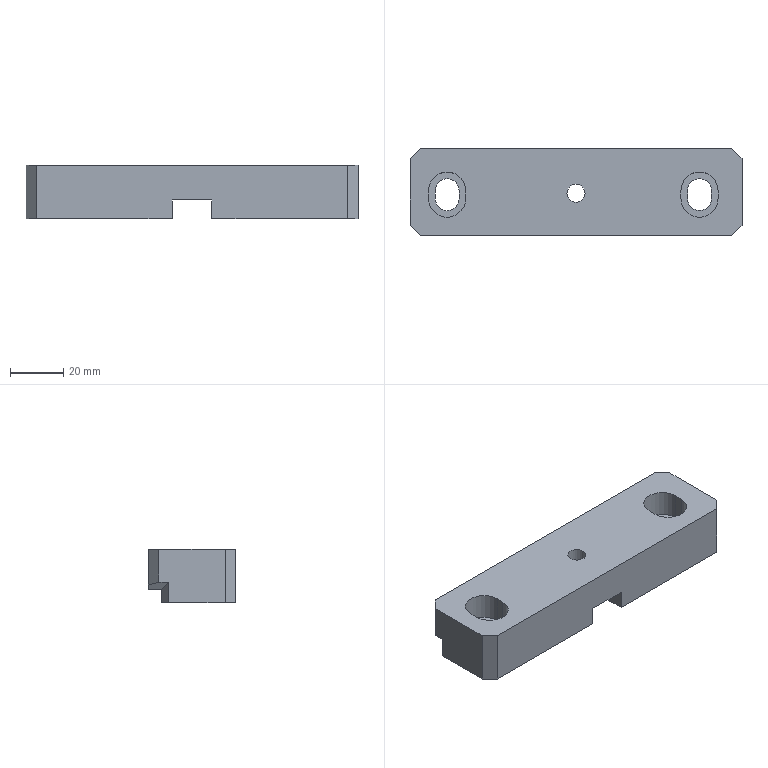Part | NX | features 20 2 | 1 solid | 46 faces | box 125 x 33 x 20 mm | volume 69012 mm3 | plane 35 | cylinder 11 | commonest cylinder face diameters 9 x4 14 x4 20 x2 6.8 x1
STEP:
#1=CARTESIAN_POINT('',(1079.502,-436.5,16.5));
#2=VERTEX_POINT('',#1);
#3=CARTESIAN_POINT('',(1079.502,-433.5,16.5));
#4=VERTEX_POINT('',#3);
#5=CARTESIAN_POINT('',(1079.502,-450.5,16.5));
#6=DIRECTION('',(0.,1.,0.));
#7=VECTOR('',#6,1000.);
#8=LINE('',#5,#7);
#9=EDGE_CURVE('',#2,#4,#8,.T.);
#10=ORIENTED_EDGE('',*,*,#9,.F.);
#11=CARTESIAN_POINT('',(1065.502,-436.5,16.5));
#12=VERTEX_POINT('',#11);
#13=CARTESIAN_POINT('',(1072.502,-436.5,16.5));
#14=DIRECTION('',(0.,0.,1.));
#15=DIRECTION('',(1.,0.,0.));
#16=AXIS2_PLACEMENT_3D('',#13,#14,#15);
#17=CIRCLE('',#16,7.);
#18=EDGE_CURVE('',#12,#2,#17,.T.);
#19=ORIENTED_EDGE('',*,*,#18,.F.);
#20=CARTESIAN_POINT('',(1065.502,-433.5,16.5));
#21=VERTEX_POINT('',#20);
#22=CARTESIAN_POINT('',(1065.502,-450.5,16.5));
#23=DIRECTION('',(0.,-1.,0.));
#24=VECTOR('',#23,1000.);
#25=LINE('',#22,#24);
#26=EDGE_CURVE('',#21,#12,#25,.T.);
#27=ORIENTED_EDGE('',*,*,#26,.F.);
#28=CARTESIAN_POINT('',(1072.502,-433.5,16.5));
#29=DIRECTION('',(0.,0.,1.));
#30=DIRECTION('',(1.,0.,0.));
#31=AXIS2_PLACEMENT_3D('',#28,#29,#30);
#32=CIRCLE('',#31,7.);
#33=EDGE_CURVE('',#4,#21,#32,.T.);
#34=ORIENTED_EDGE('',*,*,#33,.F.);
#35=EDGE_LOOP('',(#10,#19,#27,#34));
#36=FACE_BOUND('',#35,.T.);
#37=CARTESIAN_POINT('',(1183.502,-446.5,16.5));
#38=VERTEX_POINT('',#37);
#39=CARTESIAN_POINT('',(1183.502,-421.5,16.5));
#40=VERTEX_POINT('',#39);
#41=CARTESIAN_POINT('',(1183.502,-450.5,16.5));
#42=DIRECTION('',(0.,1.,0.));
#43=VECTOR('',#42,1000.);
#44=LINE('',#41,#43);
#45=EDGE_CURVE('',#38,#40,#44,.T.);
#46=ORIENTED_EDGE('',*,*,#45,.T.);
#47=CARTESIAN_POINT('',(1179.502,-417.5,16.5));
#48=VERTEX_POINT('',#47);
#49=CARTESIAN_POINT('',(1179.502,-417.5,16.5));
#50=DIRECTION('',(-0.7071,0.7071,0.));
#51=VECTOR('',#50,1000.);
#52=LINE('',#49,#51);
#53=EDGE_CURVE('',#40,#48,#52,.T.);
#54=ORIENTED_EDGE('',*,*,#53,.T.);
#55=CARTESIAN_POINT('',(1062.502,-417.5,16.5));
#56=VERTEX_POINT('',#55);
#57=CARTESIAN_POINT('',(1216.502,-417.5,16.5));
#58=DIRECTION('',(-1.,0.,0.));
#59=VECTOR('',#58,1000.);
#60=LINE('',#57,#59);
#61=EDGE_CURVE('',#48,#56,#60,.T.);
#62=ORIENTED_EDGE('',*,*,#61,.T.);
#63=CARTESIAN_POINT('',(1058.502,-421.5,16.5));
#64=VERTEX_POINT('',#63);
#65=CARTESIAN_POINT('',(1058.502,-421.5,16.5));
#66=DIRECTION('',(-0.7071,-0.7071,0.));
#67=VECTOR('',#66,1000.);
#68=LINE('',#65,#67);
#69=EDGE_CURVE('',#56,#64,#68,.T.);
#70=ORIENTED_EDGE('',*,*,#69,.T.);
#71=CARTESIAN_POINT('',(1058.502,-446.5,16.5));
#72=VERTEX_POINT('',#71);
#73=CARTESIAN_POINT('',(1058.502,-417.5,16.5));
#74=DIRECTION('',(0.,-1.,0.));
#75=VECTOR('',#74,1000.);
#76=LINE('',#73,#75);
#77=EDGE_CURVE('',#64,#72,#76,.T.);
#78=ORIENTED_EDGE('',*,*,#77,.T.);
#79=CARTESIAN_POINT('',(1062.502,-450.5,16.5));
#80=VERTEX_POINT('',#79);
#81=CARTESIAN_POINT('',(1062.502,-450.5,16.5));
#82=DIRECTION('',(0.7071,-0.7071,0.));
#83=VECTOR('',#82,1000.);
#84=LINE('',#81,#83);
#85=EDGE_CURVE('',#72,#80,#84,.T.);
#86=ORIENTED_EDGE('',*,*,#85,.T.);
#87=CARTESIAN_POINT('',(1179.502,-450.5,16.5));
#88=VERTEX_POINT('',#87);
#89=CARTESIAN_POINT('',(1136.502,-450.5,16.5));
#90=DIRECTION('',(1.,0.,0.));
#91=VECTOR('',#90,1000.);
#92=LINE('',#89,#91);
#93=EDGE_CURVE('',#80,#88,#92,.T.);
#94=ORIENTED_EDGE('',*,*,#93,.T.);
#95=CARTESIAN_POINT('',(1183.502,-446.5,16.5));
#96=DIRECTION('',(0.7071,0.7071,0.));
#97=VECTOR('',#96,1000.);
#98=LINE('',#95,#97);
#99=EDGE_CURVE('',#88,#38,#98,.T.);
#100=ORIENTED_EDGE('',*,*,#99,.T.);
#101=EDGE_LOOP('',(#46,#54,#62,#70,#78,#86,#94,#100));
#102=FACE_BOUND('',#101,.T.);
#103=CARTESIAN_POINT('',(1160.502,-433.5,16.5));
#104=VERTEX_POINT('',#103);
#105=CARTESIAN_POINT('',(1160.502,-436.5,16.5));
#106=VERTEX_POINT('',#105);
#107=CARTESIAN_POINT('',(1160.502,-450.5,16.5));
#108=DIRECTION('',(0.,-1.,0.));
#109=VECTOR('',#108,1000.);
#110=LINE('',#107,#109);
#111=EDGE_CURVE('',#104,#106,#110,.T.);
#112=ORIENTED_EDGE('',*,*,#111,.F.);
#113=CARTESIAN_POINT('',(1174.502,-433.5,16.5));
#114=VERTEX_POINT('',#113);
#115=CARTESIAN_POINT('',(1167.502,-433.5,16.5));
#116=DIRECTION('',(0.,0.,1.));
#117=DIRECTION('',(1.,0.,0.));
#118=AXIS2_PLACEMENT_3D('',#115,#116,#117);
#119=CIRCLE('',#118,7.);
#120=EDGE_CURVE('',#114,#104,#119,.T.);
#121=ORIENTED_EDGE('',*,*,#120,.F.);
#122=CARTESIAN_POINT('',(1174.502,-436.5,16.5));
#123=VERTEX_POINT('',#122);
#124=CARTESIAN_POINT('',(1174.502,-450.5,16.5));
#125=DIRECTION('',(0.,1.,0.));
#126=VECTOR('',#125,1000.);
#127=LINE('',#124,#126);
#128=EDGE_CURVE('',#123,#114,#127,.T.);
#129=ORIENTED_EDGE('',*,*,#128,.F.);
#130=CARTESIAN_POINT('',(1167.502,-436.5,16.5));
#131=DIRECTION('',(0.,0.,1.));
#132=DIRECTION('',(1.,0.,0.));
#133=AXIS2_PLACEMENT_3D('',#130,#131,#132);
#134=CIRCLE('',#133,7.);
#135=EDGE_CURVE('',#106,#123,#134,.T.);
#136=ORIENTED_EDGE('',*,*,#135,.F.);
#137=EDGE_LOOP('',(#112,#121,#129,#136));
#138=FACE_BOUND('',#137,.T.);
#139=CARTESIAN_POINT('',(1124.402,-434.5,16.5));
#140=VERTEX_POINT('',#139);
#141=CARTESIAN_POINT('',(1121.002,-434.5,16.5));
#142=DIRECTION('',(0.,0.,-1.));
#143=DIRECTION('',(1.,0.,0.));
#144=AXIS2_PLACEMENT_3D('',#141,#142,#143);
#145=CIRCLE('',#144,3.4);
#146=EDGE_CURVE('',#140,#140,#145,.T.);
#147=ORIENTED_EDGE('',*,*,#146,.T.);
#148=EDGE_LOOP('',(#147));
#149=FACE_BOUND('',#148,.T.);
#150=CARTESIAN_POINT('',(1216.502,-450.5,16.5));
#151=DIRECTION('',(0.,0.,1.));
#152=DIRECTION('',(-1.,0.,0.));
#153=AXIS2_PLACEMENT_3D('',#150,#151,#152);
#154=PLANE('',#153);
#155=ADVANCED_FACE('',(#36,#102,#138,#149),#154,.T.);
#156=CARTESIAN_POINT('',(1142.83,-427.057,-2.5));
#157=VERTEX_POINT('',#156);
#158=CARTESIAN_POINT('',(1147.07,-428.,-2.5));
#159=VERTEX_POINT('',#158);
#160=CARTESIAN_POINT('',(1147.07,-418.,-2.5));
#161=DIRECTION('',(0.,0.,1.));
#162=DIRECTION('',(1.,0.,0.));
#163=AXIS2_PLACEMENT_3D('',#160,#161,#162);
#164=CIRCLE('',#163,10.);
#165=EDGE_CURVE('',#157,#159,#164,.T.);
#166=ORIENTED_EDGE('',*,*,#165,.T.);
#167=CARTESIAN_POINT('',(1147.07,-428.,-3.5));
#168=VERTEX_POINT('',#167);
#169=CARTESIAN_POINT('',(1147.07,-428.,-43.5));
#170=DIRECTION('',(0.,0.,-1.));
#171=VECTOR('',#170,1000.);
#172=LINE('',#169,#171);
#173=EDGE_CURVE('',#159,#168,#172,.T.);
#174=ORIENTED_EDGE('',*,*,#173,.T.);
#175=CARTESIAN_POINT('',(1142.83,-427.057,-3.5));
#176=VERTEX_POINT('',#175);
#177=CARTESIAN_POINT('',(1147.07,-418.,-3.5));
#178=DIRECTION('',(0.,0.,-1.));
#179=DIRECTION('',(1.,0.,0.));
#180=AXIS2_PLACEMENT_3D('',#177,#178,#179);
#181=CIRCLE('',#180,10.);
#182=EDGE_CURVE('',#168,#176,#181,.T.);
#183=ORIENTED_EDGE('',*,*,#182,.T.);
#184=CARTESIAN_POINT('',(1142.83,-427.057,-43.5));
#185=DIRECTION('',(0.,0.,-1.));
#186=VECTOR('',#185,1000.);
#187=LINE('',#184,#186);
#188=EDGE_CURVE('',#157,#176,#187,.T.);
#189=ORIENTED_EDGE('',*,*,#188,.F.);
#190=EDGE_LOOP('',(#166,#174,#183,#189));
#191=FACE_BOUND('',#190,.T.);
#192=CARTESIAN_POINT('',(1147.07,-418.,-43.5));
#193=DIRECTION('',(0.,0.,1.));
#194=DIRECTION('',(-1.,0.,0.));
#195=AXIS2_PLACEMENT_3D('',#192,#193,#194);
#196=CYLINDRICAL_SURFACE('',#195,10.);
#197=ADVANCED_FACE('',(#191),#196,.F.);
#198=CARTESIAN_POINT('',(1133.095,-422.5,-2.5));
#199=VERTEX_POINT('',#198);
#200=CARTESIAN_POINT('',(1091.314,-402.943,-2.5));
#201=DIRECTION('',(-0.9057,0.4239,0.));
#202=VECTOR('',#201,1000.);
#203=LINE('',#200,#202);
#204=EDGE_CURVE('',#157,#199,#203,.T.);
#205=ORIENTED_EDGE('',*,*,#204,.F.);
#206=ORIENTED_EDGE('',*,*,#188,.T.);
#207=CARTESIAN_POINT('',(1133.095,-422.5,-3.5));
#208=VERTEX_POINT('',#207);
#209=CARTESIAN_POINT('',(1089.222,-401.964,-3.5));
#210=DIRECTION('',(0.9057,-0.4239,0.));
#211=VECTOR('',#210,1000.);
#212=LINE('',#209,#211);
#213=EDGE_CURVE('',#208,#176,#212,.T.);
#214=ORIENTED_EDGE('',*,*,#213,.F.);
#215=CARTESIAN_POINT('',(1133.095,-422.5,3.5));
#216=DIRECTION('',(0.,0.,-1.));
#217=VECTOR('',#216,1000.);
#218=LINE('',#215,#217);
#219=EDGE_CURVE('',#199,#208,#218,.T.);
#220=ORIENTED_EDGE('',*,*,#219,.F.);
#221=EDGE_LOOP('',(#205,#206,#214,#220));
#222=FACE_BOUND('',#221,.T.);
#223=CARTESIAN_POINT('',(1091.314,-402.943,-43.5));
#224=DIRECTION('',(-0.4239,-0.9057,0.));
#225=DIRECTION('',(-0.9057,0.4239,0.));
#226=AXIS2_PLACEMENT_3D('',#223,#224,#225);
#227=PLANE('',#226);
#228=ADVANCED_FACE('',(#222),#227,.F.);
#229=CARTESIAN_POINT('',(1183.502,-427.984,-2.5));
#230=VERTEX_POINT('',#229);
#231=CARTESIAN_POINT('',(1182.929,-428.,-2.5));
#232=VERTEX_POINT('',#231);
#233=CARTESIAN_POINT('',(1182.929,-418.,-2.5));
#234=DIRECTION('',(0.,0.,-1.));
#235=DIRECTION('',(1.,0.,0.));
#236=AXIS2_PLACEMENT_3D('',#233,#234,#235);
#237=CIRCLE('',#236,10.);
#238=EDGE_CURVE('',#230,#232,#237,.T.);
#239=ORIENTED_EDGE('',*,*,#238,.F.);
#240=CARTESIAN_POINT('',(1183.502,-427.984,-3.5));
#241=VERTEX_POINT('',#240);
#242=CARTESIAN_POINT('',(1183.502,-427.984,-43.5));
#243=DIRECTION('',(0.,0.,1.));
#244=VECTOR('',#243,1000.);
#245=LINE('',#242,#244);
#246=EDGE_CURVE('',#241,#230,#245,.T.);
#247=ORIENTED_EDGE('',*,*,#246,.F.);
#248=CARTESIAN_POINT('',(1182.929,-428.,-3.5));
#249=VERTEX_POINT('',#248);
#250=CARTESIAN_POINT('',(1182.929,-418.,-3.5));
#251=DIRECTION('',(0.,0.,1.));
#252=DIRECTION('',(1.,0.,0.));
#253=AXIS2_PLACEMENT_3D('',#250,#251,#252);
#254=CIRCLE('',#253,10.);
#255=EDGE_CURVE('',#249,#241,#254,.T.);
#256=ORIENTED_EDGE('',*,*,#255,.F.);
#257=CARTESIAN_POINT('',(1182.929,-428.,-43.5));
#258=DIRECTION('',(0.,0.,-1.));
#259=VECTOR('',#258,1000.);
#260=LINE('',#257,#259);
#261=EDGE_CURVE('',#232,#249,#260,.T.);
#262=ORIENTED_EDGE('',*,*,#261,.F.);
#263=EDGE_LOOP('',(#239,#247,#256,#262));
#264=FACE_BOUND('',#263,.T.);
#265=CARTESIAN_POINT('',(1182.929,-418.,-43.5));
#266=DIRECTION('',(0.,0.,1.));
#267=DIRECTION('',(-1.,0.,0.));
#268=AXIS2_PLACEMENT_3D('',#265,#266,#267);
#269=CYLINDRICAL_SURFACE('',#268,10.);
#270=ADVANCED_FACE('',(#264),#269,.F.);
#271=CARTESIAN_POINT('',(1163.002,-436.5,6.5));
#272=VERTEX_POINT('',#271);
#273=CARTESIAN_POINT('',(1163.002,-433.5,6.5));
#274=VERTEX_POINT('',#273);
#275=CARTESIAN_POINT('',(1163.002,-432.5,6.5));
#276=DIRECTION('',(0.,1.,0.));
#277=VECTOR('',#276,1000.);
#278=LINE('',#275,#277);
#279=EDGE_CURVE('',#272,#274,#278,.T.);
#280=ORIENTED_EDGE('',*,*,#279,.T.);
#281=CARTESIAN_POINT('',(1172.002,-433.5,6.5));
#282=VERTEX_POINT('',#281);
#283=CARTESIAN_POINT('',(1167.502,-433.5,6.5));
#284=DIRECTION('',(0.,0.,-1.));
#285=DIRECTION('',(-1.,0.,0.));
#286=AXIS2_PLACEMENT_3D('',#283,#284,#285);
#287=CIRCLE('',#286,4.5);
#288=EDGE_CURVE('',#274,#282,#287,.T.);
#289=ORIENTED_EDGE('',*,*,#288,.T.);
#290=CARTESIAN_POINT('',(1172.002,-436.5,6.5));
#291=VERTEX_POINT('',#290);
#292=CARTESIAN_POINT('',(1172.002,-439.5,6.5));
#293=DIRECTION('',(0.,-1.,0.));
#294=VECTOR('',#293,1000.);
#295=LINE('',#292,#294);
#296=EDGE_CURVE('',#282,#291,#295,.T.);
#297=ORIENTED_EDGE('',*,*,#296,.T.);
#298=CARTESIAN_POINT('',(1167.502,-436.5,6.5));
#299=DIRECTION('',(0.,0.,-1.));
#300=DIRECTION('',(-1.,0.,0.));
#301=AXIS2_PLACEMENT_3D('',#298,#299,#300);
#302=CIRCLE('',#301,4.5);
#303=EDGE_CURVE('',#291,#272,#302,.T.);
#304=ORIENTED_EDGE('',*,*,#303,.T.);
#305=EDGE_LOOP('',(#280,#289,#297,#304));
#306=FACE_BOUND('',#305,.T.);
#307=CARTESIAN_POINT('',(1174.502,-433.5,6.5));
#308=VERTEX_POINT('',#307);
#309=CARTESIAN_POINT('',(1160.502,-433.5,6.5));
#310=VERTEX_POINT('',#309);
#311=CARTESIAN_POINT('',(1167.502,-433.5,6.5));
#312=DIRECTION('',(0.,0.,1.));
#313=DIRECTION('',(-1.,0.,0.));
#314=AXIS2_PLACEMENT_3D('',#311,#312,#313);
#315=CIRCLE('',#314,7.);
#316=EDGE_CURVE('',#308,#310,#315,.T.);
#317=ORIENTED_EDGE('',*,*,#316,.T.);
#318=CARTESIAN_POINT('',(1160.502,-436.5,6.5));
#319=VERTEX_POINT('',#318);
#320=CARTESIAN_POINT('',(1160.502,-439.5,6.5));
#321=DIRECTION('',(0.,-1.,0.));
#322=VECTOR('',#321,1000.);
#323=LINE('',#320,#322);
#324=EDGE_CURVE('',#310,#319,#323,.T.);
#325=ORIENTED_EDGE('',*,*,#324,.T.);
#326=CARTESIAN_POINT('',(1174.502,-436.5,6.5));
#327=VERTEX_POINT('',#326);
#328=CARTESIAN_POINT('',(1167.502,-436.5,6.5));
#329=DIRECTION('',(0.,0.,1.));
#330=DIRECTION('',(-1.,0.,0.));
#331=AXIS2_PLACEMENT_3D('',#328,#329,#330);
#332=CIRCLE('',#331,7.);
#333=EDGE_CURVE('',#319,#327,#332,.T.);
#334=ORIENTED_EDGE('',*,*,#333,.T.);
#335=CARTESIAN_POINT('',(1174.502,-432.5,6.5));
#336=DIRECTION('',(0.,1.,0.));
#337=VECTOR('',#336,1000.);
#338=LINE('',#335,#337);
#339=EDGE_CURVE('',#327,#308,#338,.T.);
#340=ORIENTED_EDGE('',*,*,#339,.T.);
#341=EDGE_LOOP('',(#317,#325,#334,#340));
#342=FACE_BOUND('',#341,.T.);
#343=CARTESIAN_POINT('',(1167.502,-432.5,6.5));
#344=DIRECTION('',(0.,0.,-1.));
#345=DIRECTION('',(1.,0.,0.));
#346=AXIS2_PLACEMENT_3D('',#343,#344,#345);
#347=PLANE('',#346);
#348=ADVANCED_FACE('',(#306,#342),#347,.F.);
#349=CARTESIAN_POINT('',(1077.002,-433.5,6.5));
#350=VERTEX_POINT('',#349);
#351=CARTESIAN_POINT('',(1077.002,-436.5,6.5));
#352=VERTEX_POINT('',#351);
#353=CARTESIAN_POINT('',(1077.002,-432.5,6.5));
#354=DIRECTION('',(0.,-1.,0.));
#355=VECTOR('',#354,1000.);
#356=LINE('',#353,#355);
#357=EDGE_CURVE('',#350,#352,#356,.T.);
#358=ORIENTED_EDGE('',*,*,#357,.T.);
#359=CARTESIAN_POINT('',(1068.002,-436.5,6.5));
#360=VERTEX_POINT('',#359);
#361=CARTESIAN_POINT('',(1072.502,-436.5,6.5));
#362=DIRECTION('',(0.,0.,-1.));
#363=DIRECTION('',(-1.,0.,0.));
#364=AXIS2_PLACEMENT_3D('',#361,#362,#363);
#365=CIRCLE('',#364,4.5);
#366=EDGE_CURVE('',#352,#360,#365,.T.);
#367=ORIENTED_EDGE('',*,*,#366,.T.);
#368=CARTESIAN_POINT('',(1068.002,-433.5,6.5));
#369=VERTEX_POINT('',#368);
#370=CARTESIAN_POINT('',(1068.002,-439.5,6.5));
#371=DIRECTION('',(0.,1.,0.));
#372=VECTOR('',#371,1000.);
#373=LINE('',#370,#372);
#374=EDGE_CURVE('',#360,#369,#373,.T.);
#375=ORIENTED_EDGE('',*,*,#374,.T.);
#376=CARTESIAN_POINT('',(1072.502,-433.5,6.5));
#377=DIRECTION('',(0.,0.,-1.));
#378=DIRECTION('',(-1.,0.,0.));
#379=AXIS2_PLACEMENT_3D('',#376,#377,#378);
#380=CIRCLE('',#379,4.5);
#381=EDGE_CURVE('',#369,#350,#380,.T.);
#382=ORIENTED_EDGE('',*,*,#381,.T.);
#383=EDGE_LOOP('',(#358,#367,#375,#382));
#384=FACE_BOUND('',#383,.T.);
#385=CARTESIAN_POINT('',(1079.502,-433.5,6.5));
#386=VERTEX_POINT('',#385);
#387=CARTESIAN_POINT('',(1065.502,-433.5,6.5));
#388=VERTEX_POINT('',#387);
#389=CARTESIAN_POINT('',(1072.502,-433.5,6.5));
#390=DIRECTION('',(0.,0.,1.));
#391=DIRECTION('',(-1.,0.,0.));
#392=AXIS2_PLACEMENT_3D('',#389,#390,#391);
#393=CIRCLE('',#392,7.);
#394=EDGE_CURVE('',#386,#388,#393,.T.);
#395=ORIENTED_EDGE('',*,*,#394,.T.);
#396=CARTESIAN_POINT('',(1065.502,-436.5,6.5));
#397=VERTEX_POINT('',#396);
#398=CARTESIAN_POINT('',(1065.502,-432.5,6.5));
#399=DIRECTION('',(0.,-1.,0.));
#400=VECTOR('',#399,1000.);
#401=LINE('',#398,#400);
#402=EDGE_CURVE('',#388,#397,#401,.T.);
#403=ORIENTED_EDGE('',*,*,#402,.T.);
#404=CARTESIAN_POINT('',(1079.502,-436.5,6.5));
#405=VERTEX_POINT('',#404);
#406=CARTESIAN_POINT('',(1072.502,-436.5,6.5));
#407=DIRECTION('',(0.,0.,1.));
#408=DIRECTION('',(-1.,0.,0.));
#409=AXIS2_PLACEMENT_3D('',#406,#407,#408);
#410=CIRCLE('',#409,7.);
#411=EDGE_CURVE('',#397,#405,#410,.T.);
#412=ORIENTED_EDGE('',*,*,#411,.T.);
#413=CARTESIAN_POINT('',(1079.502,-439.5,6.5));
#414=DIRECTION('',(0.,1.,0.));
#415=VECTOR('',#414,1000.);
#416=LINE('',#413,#415);
#417=EDGE_CURVE('',#405,#386,#416,.T.);
#418=ORIENTED_EDGE('',*,*,#417,.T.);
#419=EDGE_LOOP('',(#395,#403,#412,#418));
#420=FACE_BOUND('',#419,.T.);
#421=CARTESIAN_POINT('',(1072.502,-432.5,6.5));
#422=DIRECTION('',(0.,0.,-1.));
#423=DIRECTION('',(-1.,0.,0.));
#424=AXIS2_PLACEMENT_3D('',#421,#422,#423);
#425=PLANE('',#424);
#426=ADVANCED_FACE('',(#384,#420),#425,.F.);
#427=ORIENTED_EDGE('',*,*,#111,.T.);
#428=CARTESIAN_POINT('',(1160.502,-436.5,42.5));
#429=DIRECTION('',(0.,0.,1.));
#430=VECTOR('',#429,1000.);
#431=LINE('',#428,#430);
#432=EDGE_CURVE('',#319,#106,#431,.T.);
#433=ORIENTED_EDGE('',*,*,#432,.F.);
#434=ORIENTED_EDGE('',*,*,#324,.F.);
#435=CARTESIAN_POINT('',(1160.502,-433.5,42.5));
#436=DIRECTION('',(0.,0.,1.));
#437=VECTOR('',#436,1000.);
#438=LINE('',#435,#437);
#439=EDGE_CURVE('',#310,#104,#438,.T.);
#440=ORIENTED_EDGE('',*,*,#439,.T.);
#441=EDGE_LOOP('',(#427,#433,#434,#440));
#442=FACE_BOUND('',#441,.T.);
#443=CARTESIAN_POINT('',(1160.502,-439.5,42.5));
#444=DIRECTION('',(-1.,0.,0.));
#445=DIRECTION('',(0.,0.,-1.));
#446=AXIS2_PLACEMENT_3D('',#443,#444,#445);
#447=PLANE('',#446);
#448=ADVANCED_FACE('',(#442),#447,.F.);
#449=ORIENTED_EDGE('',*,*,#135,.T.);
#450=CARTESIAN_POINT('',(1174.502,-436.5,42.5));
#451=DIRECTION('',(0.,0.,1.));
#452=VECTOR('',#451,1000.);
#453=LINE('',#450,#452);
#454=EDGE_CURVE('',#327,#123,#453,.T.);
#455=ORIENTED_EDGE('',*,*,#454,.F.);
#456=ORIENTED_EDGE('',*,*,#333,.F.);
#457=ORIENTED_EDGE('',*,*,#432,.T.);
#458=EDGE_LOOP('',(#449,#455,#456,#457));
#459=FACE_BOUND('',#458,.T.);
#460=CARTESIAN_POINT('',(1167.502,-436.5,42.5));
#461=DIRECTION('',(0.,0.,-1.));
#462=DIRECTION('',(1.,0.,0.));
#463=AXIS2_PLACEMENT_3D('',#460,#461,#462);
#464=CYLINDRICAL_SURFACE('',#463,7.);
#465=ADVANCED_FACE('',(#459),#464,.F.);
#466=ORIENTED_EDGE('',*,*,#128,.T.);
#467=CARTESIAN_POINT('',(1174.502,-433.5,42.5));
#468=DIRECTION('',(0.,0.,1.));
#469=VECTOR('',#468,1000.);
#470=LINE('',#467,#469);
#471=EDGE_CURVE('',#308,#114,#470,.T.);
#472=ORIENTED_EDGE('',*,*,#471,.F.);
#473=ORIENTED_EDGE('',*,*,#339,.F.);
#474=ORIENTED_EDGE('',*,*,#454,.T.);
#475=EDGE_LOOP('',(#466,#472,#473,#474));
#476=FACE_BOUND('',#475,.T.);
#477=CARTESIAN_POINT('',(1174.502,-432.5,42.5));
#478=DIRECTION('',(1.,0.,0.));
#479=DIRECTION('',(0.,0.,1.));
#480=AXIS2_PLACEMENT_3D('',#477,#478,#479);
#481=PLANE('',#480);
#482=ADVANCED_FACE('',(#476),#481,.F.);
#483=ORIENTED_EDGE('',*,*,#120,.T.);
#484=ORIENTED_EDGE('',*,*,#439,.F.);
#485=ORIENTED_EDGE('',*,*,#316,.F.);
#486=ORIENTED_EDGE('',*,*,#471,.T.);
#487=EDGE_LOOP('',(#483,#484,#485,#486));
#488=FACE_BOUND('',#487,.T.);
#489=CARTESIAN_POINT('',(1167.502,-433.5,42.5));
#490=DIRECTION('',(0.,0.,-1.));
#491=DIRECTION('',(1.,0.,0.));
#492=AXIS2_PLACEMENT_3D('',#489,#490,#491);
#493=CYLINDRICAL_SURFACE('',#492,7.);
#494=ADVANCED_FACE('',(#488),#493,.F.);
#495=ORIENTED_EDGE('',*,*,#33,.T.);
#496=CARTESIAN_POINT('',(1065.502,-433.5,42.5));
#497=DIRECTION('',(0.,0.,-1.));
#498=VECTOR('',#497,1000.);
#499=LINE('',#496,#498);
#500=EDGE_CURVE('',#21,#388,#499,.T.);
#501=ORIENTED_EDGE('',*,*,#500,.T.);
#502=ORIENTED_EDGE('',*,*,#394,.F.);
#503=CARTESIAN_POINT('',(1079.502,-433.5,42.5));
#504=DIRECTION('',(0.,0.,-1.));
#505=VECTOR('',#504,1000.);
#506=LINE('',#503,#505);
#507=EDGE_CURVE('',#4,#386,#506,.T.);
#508=ORIENTED_EDGE('',*,*,#507,.F.);
#509=EDGE_LOOP('',(#495,#501,#502,#508));
#510=FACE_BOUND('',#509,.T.);
#511=CARTESIAN_POINT('',(1072.502,-433.5,42.5));
#512=DIRECTION('',(0.,0.,-1.));
#513=DIRECTION('',(-1.,0.,0.));
#514=AXIS2_PLACEMENT_3D('',#511,#512,#513);
#515=CYLINDRICAL_SURFACE('',#514,7.);
#516=ADVANCED_FACE('',(#510),#515,.F.);
#517=ORIENTED_EDGE('',*,*,#26,.T.);
#518=CARTESIAN_POINT('',(1065.502,-436.5,42.5));
#519=DIRECTION('',(0.,0.,-1.));
#520=VECTOR('',#519,1000.);
#521=LINE('',#518,#520);
#522=EDGE_CURVE('',#12,#397,#521,.T.);
#523=ORIENTED_EDGE('',*,*,#522,.T.);
#524=ORIENTED_EDGE('',*,*,#402,.F.);
#525=ORIENTED_EDGE('',*,*,#500,.F.);
#526=EDGE_LOOP('',(#517,#523,#524,#525));
#527=FACE_BOUND('',#526,.T.);
#528=CARTESIAN_POINT('',(1065.502,-432.5,42.5));
#529=DIRECTION('',(-1.,0.,0.));
#530=DIRECTION('',(0.,0.,1.));
#531=AXIS2_PLACEMENT_3D('',#528,#529,#530);
#532=PLANE('',#531);
#533=ADVANCED_FACE('',(#527),#532,.F.);
#534=ORIENTED_EDGE('',*,*,#18,.T.);
#535=CARTESIAN_POINT('',(1079.502,-436.5,42.5));
#536=DIRECTION('',(0.,0.,-1.));
#537=VECTOR('',#536,1000.);
#538=LINE('',#535,#537);
#539=EDGE_CURVE('',#2,#405,#538,.T.);
#540=ORIENTED_EDGE('',*,*,#539,.T.);
#541=ORIENTED_EDGE('',*,*,#411,.F.);
#542=ORIENTED_EDGE('',*,*,#522,.F.);
#543=EDGE_LOOP('',(#534,#540,#541,#542));
#544=FACE_BOUND('',#543,.T.);
#545=CARTESIAN_POINT('',(1072.502,-436.5,42.5));
#546=DIRECTION('',(0.,0.,-1.));
#547=DIRECTION('',(-1.,0.,0.));
#548=AXIS2_PLACEMENT_3D('',#545,#546,#547);
#549=CYLINDRICAL_SURFACE('',#548,7.);
#550=ADVANCED_FACE('',(#544),#549,.F.);
#551=ORIENTED_EDGE('',*,*,#9,.T.);
#552=ORIENTED_EDGE('',*,*,#507,.T.);
#553=ORIENTED_EDGE('',*,*,#417,.F.);
#554=ORIENTED_EDGE('',*,*,#539,.F.);
#555=EDGE_LOOP('',(#551,#552,#553,#554));
#556=FACE_BOUND('',#555,.T.);
#557=CARTESIAN_POINT('',(1079.502,-439.5,42.5));
#558=DIRECTION('',(1.,0.,0.));
#559=DIRECTION('',(0.,0.,-1.));
#560=AXIS2_PLACEMENT_3D('',#557,#558,#559);
#561=PLANE('',#560);
#562=ADVANCED_FACE('',(#556),#561,.F.);
#563=CARTESIAN_POINT('',(1183.502,-446.5,-3.5));
#564=VERTEX_POINT('',#563);
#565=CARTESIAN_POINT('',(1183.502,-450.5,-3.5));
#566=DIRECTION('',(0.,1.,0.));
#567=VECTOR('',#566,1000.);
#568=LINE('',#565,#567);
#569=EDGE_CURVE('',#564,#241,#568,.T.);
#570=ORIENTED_EDGE('',*,*,#569,.T.);
#571=ORIENTED_EDGE('',*,*,#246,.T.);
#572=CARTESIAN_POINT('',(1183.502,-425.18,-2.5));
#573=VERTEX_POINT('',#572);
#574=CARTESIAN_POINT('',(1183.502,-450.5,-2.5));
#575=DIRECTION('',(0.,1.,0.));
#576=VECTOR('',#575,1000.);
#577=LINE('',#574,#576);
#578=EDGE_CURVE('',#230,#573,#577,.T.);
#579=ORIENTED_EDGE('',*,*,#578,.T.);
#580=CARTESIAN_POINT('',(1183.502,-425.18,4.179));
#581=VERTEX_POINT('',#580);
#582=CARTESIAN_POINT('',(1183.502,-425.18,3.5));
#583=DIRECTION('',(0.,0.,-1.));
#584=VECTOR('',#583,1000.);
#585=LINE('',#582,#584);
#586=EDGE_CURVE('',#581,#573,#585,.T.);
#587=ORIENTED_EDGE('',*,*,#586,.F.);
#588=CARTESIAN_POINT('',(1183.502,-421.5,4.179));
#589=VERTEX_POINT('',#588);
#590=CARTESIAN_POINT('',(1183.502,-417.5,4.179));
#591=DIRECTION('',(0.,1.,0.));
#592=VECTOR('',#591,1000.);
#593=LINE('',#590,#592);
#594=EDGE_CURVE('',#581,#589,#593,.T.);
#595=ORIENTED_EDGE('',*,*,#594,.T.);
#596=CARTESIAN_POINT('',(1183.502,-421.5,11.5));
#597=DIRECTION('',(0.,0.,1.));
#598=VECTOR('',#597,1000.);
#599=LINE('',#596,#598);
#600=EDGE_CURVE('',#589,#40,#599,.T.);
#601=ORIENTED_EDGE('',*,*,#600,.T.);
#602=ORIENTED_EDGE('',*,*,#45,.F.);
#603=CARTESIAN_POINT('',(1183.502,-446.5,11.5));
#604=DIRECTION('',(0.,0.,-1.));
#605=VECTOR('',#604,1000.);
#606=LINE('',#603,#605);
#607=EDGE_CURVE('',#38,#564,#606,.T.);
#608=ORIENTED_EDGE('',*,*,#607,.T.);
#609=EDGE_LOOP('',(#570,#571,#579,#587,#595,#601,#602,#608));
#610=FACE_BOUND('',#609,.T.);
#611=CARTESIAN_POINT('',(1183.502,-450.5,11.5));
#612=DIRECTION('',(-1.,0.,0.));
#613=DIRECTION('',(0.,0.,-1.));
#614=AXIS2_PLACEMENT_3D('',#611,#612,#613);
#615=PLANE('',#614);
#616=ADVANCED_FACE('',(#610),#615,.F.);
#617=ORIENTED_EDGE('',*,*,#288,.F.);
#618=CARTESIAN_POINT('',(1163.002,-433.5,-3.5));
#619=VERTEX_POINT('',#618);
#620=CARTESIAN_POINT('',(1163.002,-433.5,42.5));
#621=DIRECTION('',(0.,0.,1.));
#622=VECTOR('',#621,1000.);
#623=LINE('',#620,#622);
#624=EDGE_CURVE('',#619,#274,#623,.T.);
#625=ORIENTED_EDGE('',*,*,#624,.F.);
#626=CARTESIAN_POINT('',(1172.002,-433.5,-3.5));
#627=VERTEX_POINT('',#626);
#628=CARTESIAN_POINT('',(1167.502,-433.5,-3.5));
#629=DIRECTION('',(0.,0.,1.));
#630=DIRECTION('',(1.,0.,0.));
#631=AXIS2_PLACEMENT_3D('',#628,#629,#630);
#632=CIRCLE('',#631,4.5);
#633=EDGE_CURVE('',#627,#619,#632,.T.);
#634=ORIENTED_EDGE('',*,*,#633,.F.);
#635=CARTESIAN_POINT('',(1172.002,-433.5,42.5));
#636=DIRECTION('',(0.,0.,1.));
#637=VECTOR('',#636,1000.);
#638=LINE('',#635,#637);
#639=EDGE_CURVE('',#627,#282,#638,.T.);
#640=ORIENTED_EDGE('',*,*,#639,.T.);
#641=EDGE_LOOP('',(#617,#625,#634,#640));
#642=FACE_BOUND('',#641,.T.);
#643=CARTESIAN_POINT('',(1167.502,-433.5,42.5));
#644=DIRECTION('',(0.,0.,-1.));
#645=DIRECTION('',(1.,0.,0.));
#646=AXIS2_PLACEMENT_3D('',#643,#644,#645);
#647=CYLINDRICAL_SURFACE('',#646,4.5);
#648=ADVANCED_FACE('',(#642),#647,.F.);
#649=ORIENTED_EDGE('',*,*,#296,.F.);
#650=ORIENTED_EDGE('',*,*,#639,.F.);
#651=CARTESIAN_POINT('',(1172.002,-436.5,-3.5));
#652=VERTEX_POINT('',#651);
#653=CARTESIAN_POINT('',(1172.002,-439.5,-3.5));
#654=DIRECTION('',(0.,1.,0.));
#655=VECTOR('',#654,1000.);
#656=LINE('',#653,#655);
#657=EDGE_CURVE('',#652,#627,#656,.T.);
#658=ORIENTED_EDGE('',*,*,#657,.F.);
#659=CARTESIAN_POINT('',(1172.002,-436.5,42.5));
#660=DIRECTION('',(0.,0.,1.));
#661=VECTOR('',#660,1000.);
#662=LINE('',#659,#661);
#663=EDGE_CURVE('',#652,#291,#662,.T.);
#664=ORIENTED_EDGE('',*,*,#663,.T.);
#665=EDGE_LOOP('',(#649,#650,#658,#664));
#666=FACE_BOUND('',#665,.T.);
#667=CARTESIAN_POINT('',(1172.002,-439.5,42.5));
#668=DIRECTION('',(-1.,0.,0.));
#669=DIRECTION('',(0.,0.,-1.));
#670=AXIS2_PLACEMENT_3D('',#667,#668,#669);
#671=PLANE('',#670);
#672=ADVANCED_FACE('',(#666),#671,.T.);
#673=ORIENTED_EDGE('',*,*,#303,.F.);
#674=ORIENTED_EDGE('',*,*,#663,.F.);
#675=CARTESIAN_POINT('',(1163.002,-436.5,-3.5));
#676=VERTEX_POINT('',#675);
#677=CARTESIAN_POINT('',(1167.502,-436.5,-3.5));
#678=DIRECTION('',(0.,0.,1.));
#679=DIRECTION('',(1.,0.,0.));
#680=AXIS2_PLACEMENT_3D('',#677,#678,#679);
#681=CIRCLE('',#680,4.5);
#682=EDGE_CURVE('',#676,#652,#681,.T.);
#683=ORIENTED_EDGE('',*,*,#682,.F.);
#684=CARTESIAN_POINT('',(1163.002,-436.5,42.5));
#685=DIRECTION('',(0.,0.,1.));
#686=VECTOR('',#685,1000.);
#687=LINE('',#684,#686);
#688=EDGE_CURVE('',#676,#272,#687,.T.);
#689=ORIENTED_EDGE('',*,*,#688,.T.);
#690=EDGE_LOOP('',(#673,#674,#683,#689));
#691=FACE_BOUND('',#690,.T.);
#692=CARTESIAN_POINT('',(1167.502,-436.5,42.5));
#693=DIRECTION('',(0.,0.,-1.));
#694=DIRECTION('',(1.,0.,0.));
#695=AXIS2_PLACEMENT_3D('',#692,#693,#694);
#696=CYLINDRICAL_SURFACE('',#695,4.5);
#697=ADVANCED_FACE('',(#691),#696,.F.);
#698=ORIENTED_EDGE('',*,*,#279,.F.);
#699=ORIENTED_EDGE('',*,*,#688,.F.);
#700=CARTESIAN_POINT('',(1163.002,-432.5,-3.5));
#701=DIRECTION('',(0.,-1.,0.));
#702=VECTOR('',#701,1000.);
#703=LINE('',#700,#702);
#704=EDGE_CURVE('',#619,#676,#703,.T.);
#705=ORIENTED_EDGE('',*,*,#704,.F.);
#706=ORIENTED_EDGE('',*,*,#624,.T.);
#707=EDGE_LOOP('',(#698,#699,#705,#706));
#708=FACE_BOUND('',#707,.T.);
#709=CARTESIAN_POINT('',(1163.002,-432.5,42.5));
#710=DIRECTION('',(1.,0.,0.));
#711=DIRECTION('',(0.,0.,1.));
#712=AXIS2_PLACEMENT_3D('',#709,#710,#711);
#713=PLANE('',#712);
#714=ADVANCED_FACE('',(#708),#713,.T.);
#715=CARTESIAN_POINT('',(1128.502,-422.5,1.5));
#716=VERTEX_POINT('',#715);
#717=CARTESIAN_POINT('',(1173.501,-422.5,1.5));
#718=VERTEX_POINT('',#717);
#719=CARTESIAN_POINT('',(1098.773,-422.5,1.5));
#720=DIRECTION('',(1.,0.,0.));
#721=VECTOR('',#720,1000.);
#722=LINE('',#719,#721);
#723=EDGE_CURVE('',#716,#718,#722,.T.);
#724=ORIENTED_EDGE('',*,*,#723,.T.);
#725=CARTESIAN_POINT('',(1173.501,-422.5,-2.5));
#726=VERTEX_POINT('',#725);
#727=CARTESIAN_POINT('',(1173.501,-422.5,3.5));
#728=DIRECTION('',(0.,0.,1.));
#729=VECTOR('',#728,1000.);
#730=LINE('',#727,#729);
#731=EDGE_CURVE('',#726,#718,#730,.T.);
#732=ORIENTED_EDGE('',*,*,#731,.F.);
#733=CARTESIAN_POINT('',(1116.501,-422.5,-2.5));
#734=DIRECTION('',(-1.,0.,0.));
#735=VECTOR('',#734,1000.);
#736=LINE('',#733,#735);
#737=EDGE_CURVE('',#726,#199,#736,.T.);
#738=ORIENTED_EDGE('',*,*,#737,.T.);
#739=ORIENTED_EDGE('',*,*,#219,.T.);
#740=CARTESIAN_POINT('',(1128.502,-422.5,-3.5));
#741=VERTEX_POINT('',#740);
#742=CARTESIAN_POINT('',(1116.501,-422.5,-3.5));
#743=DIRECTION('',(-1.,0.,0.));
#744=VECTOR('',#743,1000.);
#745=LINE('',#742,#744);
#746=EDGE_CURVE('',#208,#741,#745,.T.);
#747=ORIENTED_EDGE('',*,*,#746,.T.);
#748=CARTESIAN_POINT('',(1128.502,-422.5,-9.5));
#749=DIRECTION('',(0.,0.,1.));
#750=VECTOR('',#749,1000.);
#751=LINE('',#748,#750);
#752=EDGE_CURVE('',#741,#716,#751,.T.);
#753=ORIENTED_EDGE('',*,*,#752,.T.);
#754=EDGE_LOOP('',(#724,#732,#738,#739,#747,#753));
#755=FACE_BOUND('',#754,.T.);
#756=CARTESIAN_POINT('',(1116.501,-422.5,3.5));
#757=DIRECTION('',(0.,-1.,0.));
#758=DIRECTION('',(0.,0.,1.));
#759=AXIS2_PLACEMENT_3D('',#756,#757,#758);
#760=PLANE('',#759);
#761=ADVANCED_FACE('',(#755),#760,.F.);
#762=CARTESIAN_POINT('',(1128.502,-417.5,1.5));
#763=VERTEX_POINT('',#762);
#764=CARTESIAN_POINT('',(1128.502,-436.5,1.5));
#765=DIRECTION('',(0.,1.,0.));
#766=VECTOR('',#765,1000.);
#767=LINE('',#764,#766);
#768=EDGE_CURVE('',#716,#763,#767,.T.);
#769=ORIENTED_EDGE('',*,*,#768,.T.);
#770=CARTESIAN_POINT('',(1173.502,-417.5,1.5));
#771=VERTEX_POINT('',#770);
#772=CARTESIAN_POINT('',(1076.502,-417.5,1.5));
#773=DIRECTION('',(1.,0.,0.));
#774=VECTOR('',#773,1000.);
#775=LINE('',#772,#774);
#776=EDGE_CURVE('',#763,#771,#775,.T.);
#777=ORIENTED_EDGE('',*,*,#776,.T.);
#778=CARTESIAN_POINT('',(1173.502,-422.5,1.5));
#779=VERTEX_POINT('',#778);
#780=CARTESIAN_POINT('',(1173.502,-425.18,1.5));
#781=DIRECTION('',(0.,-1.,0.));
#782=VECTOR('',#781,1000.);
#783=LINE('',#780,#782);
#784=EDGE_CURVE('',#771,#779,#783,.T.);
#785=ORIENTED_EDGE('',*,*,#784,.T.);
#786=CARTESIAN_POINT('',(1183.502,-425.18,1.5));
#787=DIRECTION('',(0.9659,-0.2588,0.));
#788=VECTOR('',#787,1000.);
#789=LINE('',#786,#788);
#790=EDGE_CURVE('',#718,#779,#789,.T.);
#791=ORIENTED_EDGE('',*,*,#790,.F.);
#792=ORIENTED_EDGE('',*,*,#723,.F.);
#793=EDGE_LOOP('',(#769,#777,#785,#791,#792));
#794=FACE_BOUND('',#793,.T.);
#795=CARTESIAN_POINT('',(1148.773,-396.891,1.5));
#796=DIRECTION('',(0.,0.,-1.));
#797=DIRECTION('',(1.,0.,0.));
#798=AXIS2_PLACEMENT_3D('',#795,#796,#797);
#799=PLANE('',#798);
#800=ADVANCED_FACE('',(#794),#799,.T.);
#801=ORIENTED_EDGE('',*,*,#61,.F.);
#802=CARTESIAN_POINT('',(1179.502,-417.5,3.108));
#803=VERTEX_POINT('',#802);
#804=CARTESIAN_POINT('',(1179.502,-417.5,11.5));
#805=DIRECTION('',(0.,0.,-1.));
#806=VECTOR('',#805,1000.);
#807=LINE('',#804,#806);
#808=EDGE_CURVE('',#48,#803,#807,.T.);
#809=ORIENTED_EDGE('',*,*,#808,.T.);
#810=CARTESIAN_POINT('',(1173.502,-417.5,1.5));
#811=DIRECTION('',(-0.9659,0.,-0.2588));
#812=VECTOR('',#811,1000.);
#813=LINE('',#810,#812);
#814=EDGE_CURVE('',#803,#771,#813,.T.);
#815=ORIENTED_EDGE('',*,*,#814,.T.);
#816=ORIENTED_EDGE('',*,*,#776,.F.);
#817=CARTESIAN_POINT('',(1128.502,-417.5,3.5));
#818=VERTEX_POINT('',#817);
#819=CARTESIAN_POINT('',(1128.502,-417.5,11.5));
#820=DIRECTION('',(0.,0.,-1.));
#821=VECTOR('',#820,1000.);
#822=LINE('',#819,#821);
#823=EDGE_CURVE('',#818,#763,#822,.T.);
#824=ORIENTED_EDGE('',*,*,#823,.F.);
#825=CARTESIAN_POINT('',(1113.502,-417.5,3.5));
#826=VERTEX_POINT('',#825);
#827=CARTESIAN_POINT('',(1104.002,-417.5,3.5));
#828=DIRECTION('',(1.,0.,0.));
#829=VECTOR('',#828,1000.);
#830=LINE('',#827,#829);
#831=EDGE_CURVE('',#826,#818,#830,.T.);
#832=ORIENTED_EDGE('',*,*,#831,.F.);
#833=CARTESIAN_POINT('',(1113.502,-417.5,1.5));
#834=VERTEX_POINT('',#833);
#835=CARTESIAN_POINT('',(1113.502,-417.5,11.5));
#836=DIRECTION('',(0.,0.,1.));
#837=VECTOR('',#836,1000.);
#838=LINE('',#835,#837);
#839=EDGE_CURVE('',#834,#826,#838,.T.);
#840=ORIENTED_EDGE('',*,*,#839,.F.);
#841=CARTESIAN_POINT('',(1068.502,-417.5,1.5));
#842=VERTEX_POINT('',#841);
#843=CARTESIAN_POINT('',(1194.502,-417.5,1.5));
#844=DIRECTION('',(1.,0.,0.));
#845=VECTOR('',#844,1000.);
#846=LINE('',#843,#845);
#847=EDGE_CURVE('',#842,#834,#846,.T.);
#848=ORIENTED_EDGE('',*,*,#847,.F.);
#849=CARTESIAN_POINT('',(1062.502,-417.5,3.108));
#850=VERTEX_POINT('',#849);
#851=CARTESIAN_POINT('',(1068.502,-417.5,1.5));
#852=DIRECTION('',(-0.9659,0.,0.2588));
#853=VECTOR('',#852,1000.);
#854=LINE('',#851,#853);
#855=EDGE_CURVE('',#842,#850,#854,.T.);
#856=ORIENTED_EDGE('',*,*,#855,.T.);
#857=CARTESIAN_POINT('',(1062.502,-417.5,11.5));
#858=DIRECTION('',(0.,0.,1.));
#859=VECTOR('',#858,1000.);
#860=LINE('',#857,#859);
#861=EDGE_CURVE('',#850,#56,#860,.T.);
#862=ORIENTED_EDGE('',*,*,#861,.T.);
#863=EDGE_LOOP('',(#801,#809,#815,#816,#824,#832,#840,#848,#856,#862));
#864=FACE_BOUND('',#863,.T.);
#865=CARTESIAN_POINT('',(1216.502,-417.5,11.5));
#866=DIRECTION('',(0.,-1.,0.));
#867=DIRECTION('',(0.,0.,1.));
#868=AXIS2_PLACEMENT_3D('',#865,#866,#867);
#869=PLANE('',#868);
#870=ADVANCED_FACE('',(#864),#869,.F.);
#871=ORIENTED_EDGE('',*,*,#69,.F.);
#872=ORIENTED_EDGE('',*,*,#861,.F.);
#873=CARTESIAN_POINT('',(1058.502,-421.5,4.179));
#874=VERTEX_POINT('',#873);
#875=CARTESIAN_POINT('',(1075.554,-404.449,-0.3894));
#876=DIRECTION('',(0.6947,0.6947,-0.1862));
#877=VECTOR('',#876,1000.);
#878=LINE('',#875,#877);
#879=EDGE_CURVE('',#874,#850,#878,.T.);
#880=ORIENTED_EDGE('',*,*,#879,.F.);
#881=CARTESIAN_POINT('',(1058.502,-421.5,11.5));
#882=DIRECTION('',(0.,0.,-1.));
#883=VECTOR('',#882,1000.);
#884=LINE('',#881,#883);
#885=EDGE_CURVE('',#64,#874,#884,.T.);
#886=ORIENTED_EDGE('',*,*,#885,.F.);
#887=EDGE_LOOP('',(#871,#872,#880,#886));
#888=FACE_BOUND('',#887,.T.);
#889=CARTESIAN_POINT('',(1058.502,-421.5,11.5));
#890=DIRECTION('',(0.7071,-0.7071,0.));
#891=DIRECTION('',(0.,0.,-1.));
#892=AXIS2_PLACEMENT_3D('',#889,#890,#891);
#893=PLANE('',#892);
#894=ADVANCED_FACE('',(#888),#893,.F.);
#895=ORIENTED_EDGE('',*,*,#366,.F.);
#896=CARTESIAN_POINT('',(1077.002,-436.5,-3.5));
#897=VERTEX_POINT('',#896);
#898=CARTESIAN_POINT('',(1077.002,-436.5,42.5));
#899=DIRECTION('',(0.,0.,-1.));
#900=VECTOR('',#899,1000.);
#901=LINE('',#898,#900);
#902=EDGE_CURVE('',#352,#897,#901,.T.);
#903=ORIENTED_EDGE('',*,*,#902,.T.);
#904=CARTESIAN_POINT('',(1068.002,-436.5,-3.5));
#905=VERTEX_POINT('',#904);
#906=CARTESIAN_POINT('',(1072.502,-436.5,-3.5));
#907=DIRECTION('',(0.,0.,-1.));
#908=DIRECTION('',(1.,0.,0.));
#909=AXIS2_PLACEMENT_3D('',#906,#907,#908);
#910=CIRCLE('',#909,4.5);
#911=EDGE_CURVE('',#897,#905,#910,.T.);
#912=ORIENTED_EDGE('',*,*,#911,.T.);
#913=CARTESIAN_POINT('',(1068.002,-436.5,42.5));
#914=DIRECTION('',(0.,0.,-1.));
#915=VECTOR('',#914,1000.);
#916=LINE('',#913,#915);
#917=EDGE_CURVE('',#360,#905,#916,.T.);
#918=ORIENTED_EDGE('',*,*,#917,.F.);
#919=EDGE_LOOP('',(#895,#903,#912,#918));
#920=FACE_BOUND('',#919,.T.);
#921=CARTESIAN_POINT('',(1072.502,-436.5,42.5));
#922=DIRECTION('',(0.,0.,-1.));
#923=DIRECTION('',(-1.,0.,0.));
#924=AXIS2_PLACEMENT_3D('',#921,#922,#923);
#925=CYLINDRICAL_SURFACE('',#924,4.5);
#926=ADVANCED_FACE('',(#920),#925,.F.);
#927=ORIENTED_EDGE('',*,*,#374,.F.);
#928=ORIENTED_EDGE('',*,*,#917,.T.);
#929=CARTESIAN_POINT('',(1068.002,-433.5,-3.5));
#930=VERTEX_POINT('',#929);
#931=CARTESIAN_POINT('',(1068.002,-450.5,-3.5));
#932=DIRECTION('',(0.,1.,0.));
#933=VECTOR('',#932,1000.);
#934=LINE('',#931,#933);
#935=EDGE_CURVE('',#905,#930,#934,.T.);
#936=ORIENTED_EDGE('',*,*,#935,.T.);
#937=CARTESIAN_POINT('',(1068.002,-433.5,42.5));
#938=DIRECTION('',(0.,0.,-1.));
#939=VECTOR('',#938,1000.);
#940=LINE('',#937,#939);
#941=EDGE_CURVE('',#369,#930,#940,.T.);
#942=ORIENTED_EDGE('',*,*,#941,.F.);
#943=EDGE_LOOP('',(#927,#928,#936,#942));
#944=FACE_BOUND('',#943,.T.);
#945=CARTESIAN_POINT('',(1068.002,-439.5,42.5));
#946=DIRECTION('',(1.,0.,0.));
#947=DIRECTION('',(0.,0.,-1.));
#948=AXIS2_PLACEMENT_3D('',#945,#946,#947);
#949=PLANE('',#948);
#950=ADVANCED_FACE('',(#944),#949,.T.);
#951=ORIENTED_EDGE('',*,*,#381,.F.);
#952=ORIENTED_EDGE('',*,*,#941,.T.);
#953=CARTESIAN_POINT('',(1077.002,-433.5,-3.5));
#954=VERTEX_POINT('',#953);
#955=CARTESIAN_POINT('',(1072.502,-433.5,-3.5));
#956=DIRECTION('',(0.,0.,-1.));
#957=DIRECTION('',(1.,0.,0.));
#958=AXIS2_PLACEMENT_3D('',#955,#956,#957);
#959=CIRCLE('',#958,4.5);
#960=EDGE_CURVE('',#930,#954,#959,.T.);
#961=ORIENTED_EDGE('',*,*,#960,.T.);
#962=CARTESIAN_POINT('',(1077.002,-433.5,42.5));
#963=DIRECTION('',(0.,0.,-1.));
#964=VECTOR('',#963,1000.);
#965=LINE('',#962,#964);
#966=EDGE_CURVE('',#350,#954,#965,.T.);
#967=ORIENTED_EDGE('',*,*,#966,.F.);
#968=EDGE_LOOP('',(#951,#952,#961,#967));
#969=FACE_BOUND('',#968,.T.);
#970=CARTESIAN_POINT('',(1072.502,-433.5,42.5));
#971=DIRECTION('',(0.,0.,-1.));
#972=DIRECTION('',(-1.,0.,0.));
#973=AXIS2_PLACEMENT_3D('',#970,#971,#972);
#974=CYLINDRICAL_SURFACE('',#973,4.5);
#975=ADVANCED_FACE('',(#969),#974,.F.);
#976=ORIENTED_EDGE('',*,*,#357,.F.);
#977=ORIENTED_EDGE('',*,*,#966,.T.);
#978=CARTESIAN_POINT('',(1077.002,-450.5,-3.5));
#979=DIRECTION('',(0.,-1.,0.));
#980=VECTOR('',#979,1000.);
#981=LINE('',#978,#980);
#982=EDGE_CURVE('',#954,#897,#981,.T.);
#983=ORIENTED_EDGE('',*,*,#982,.T.);
#984=ORIENTED_EDGE('',*,*,#902,.F.);
#985=EDGE_LOOP('',(#976,#977,#983,#984));
#986=FACE_BOUND('',#985,.T.);
#987=CARTESIAN_POINT('',(1077.002,-432.5,42.5));
#988=DIRECTION('',(-1.,0.,0.));
#989=DIRECTION('',(0.,0.,1.));
#990=AXIS2_PLACEMENT_3D('',#987,#988,#989);
#991=PLANE('',#990);
#992=ADVANCED_FACE('',(#986),#991,.T.);
#993=ORIENTED_EDGE('',*,*,#77,.F.);
#994=ORIENTED_EDGE('',*,*,#885,.T.);
#995=CARTESIAN_POINT('',(1058.502,-425.179,4.179));
#996=VERTEX_POINT('',#995);
#997=CARTESIAN_POINT('',(1058.502,-425.179,4.179));
#998=DIRECTION('',(0.,-1.,0.));
#999=VECTOR('',#998,1000.);
#1000=LINE('',#997,#999);
#1001=EDGE_CURVE('',#874,#996,#1000,.T.);
#1002=ORIENTED_EDGE('',*,*,#1001,.T.);
#1003=CARTESIAN_POINT('',(1058.502,-425.179,-3.5));
#1004=VERTEX_POINT('',#1003);
#1005=CARTESIAN_POINT('',(1058.502,-425.179,3.5));
#1006=DIRECTION('',(0.,0.,-1.));
#1007=VECTOR('',#1006,1000.);
#1008=LINE('',#1005,#1007);
#1009=EDGE_CURVE('',#996,#1004,#1008,.T.);
#1010=ORIENTED_EDGE('',*,*,#1009,.T.);
#1011=CARTESIAN_POINT('',(1058.502,-446.5,-3.5));
#1012=VERTEX_POINT('',#1011);
#1013=CARTESIAN_POINT('',(1058.502,-417.5,-3.5));
#1014=DIRECTION('',(0.,-1.,0.));
#1015=VECTOR('',#1014,1000.);
#1016=LINE('',#1013,#1015);
#1017=EDGE_CURVE('',#1004,#1012,#1016,.T.);
#1018=ORIENTED_EDGE('',*,*,#1017,.T.);
#1019=CARTESIAN_POINT('',(1058.502,-446.5,11.5));
#1020=DIRECTION('',(0.,0.,1.));
#1021=VECTOR('',#1020,1000.);
#1022=LINE('',#1019,#1021);
#1023=EDGE_CURVE('',#1012,#72,#1022,.T.);
#1024=ORIENTED_EDGE('',*,*,#1023,.T.);
#1025=EDGE_LOOP('',(#993,#994,#1002,#1010,#1018,#1024));
#1026=FACE_BOUND('',#1025,.T.);
#1027=CARTESIAN_POINT('',(1058.502,-417.5,11.5));
#1028=DIRECTION('',(1.,0.,0.));
#1029=DIRECTION('',(0.,0.,1.));
#1030=AXIS2_PLACEMENT_3D('',#1027,#1028,#1029);
#1031=PLANE('',#1030);
#1032=ADVANCED_FACE('',(#1026),#1031,.F.);
#1033=ORIENTED_EDGE('',*,*,#1001,.F.);
#1034=ORIENTED_EDGE('',*,*,#879,.T.);
#1035=ORIENTED_EDGE('',*,*,#855,.F.);
#1036=CARTESIAN_POINT('',(1068.502,-422.5,1.5));
#1037=VERTEX_POINT('',#1036);
#1038=CARTESIAN_POINT('',(1068.502,-417.5,1.5));
#1039=DIRECTION('',(0.,1.,0.));
#1040=VECTOR('',#1039,1000.);
#1041=LINE('',#1038,#1040);
#1042=EDGE_CURVE('',#1037,#842,#1041,.T.);
#1043=ORIENTED_EDGE('',*,*,#1042,.F.);
#1044=CARTESIAN_POINT('',(1068.501,-422.5,1.5));
#1045=VERTEX_POINT('',#1044);
#1046=CARTESIAN_POINT('',(1068.502,-422.5,1.5));
#1047=DIRECTION('',(0.9659,0.,-0.2588));
#1048=VECTOR('',#1047,1000.);
#1049=LINE('',#1046,#1048);
#1050=EDGE_CURVE('',#1045,#1037,#1049,.T.);
#1051=ORIENTED_EDGE('',*,*,#1050,.F.);
#1052=CARTESIAN_POINT('',(1068.501,-422.5,1.5));
#1053=DIRECTION('',(0.9351,0.2506,-0.2506));
#1054=VECTOR('',#1053,1000.);
#1055=LINE('',#1052,#1054);
#1056=EDGE_CURVE('',#996,#1045,#1055,.T.);
#1057=ORIENTED_EDGE('',*,*,#1056,.F.);
#1058=EDGE_LOOP('',(#1033,#1034,#1035,#1043,#1051,#1057));
#1059=FACE_BOUND('',#1058,.T.);
#1060=CARTESIAN_POINT('',(1068.502,-396.891,1.5));
#1061=DIRECTION('',(-0.2588,0.,-0.9659));
#1062=DIRECTION('',(0.9659,0.,-0.2588));
#1063=AXIS2_PLACEMENT_3D('',#1060,#1061,#1062);
#1064=PLANE('',#1063);
#1065=ADVANCED_FACE('',(#1059),#1064,.T.);
#1066=CARTESIAN_POINT('',(1068.501,-422.5,-3.5));
#1067=VERTEX_POINT('',#1066);
#1068=CARTESIAN_POINT('',(1068.501,-422.5,-3.5));
#1069=DIRECTION('',(-0.9659,-0.2588,0.));
#1070=VECTOR('',#1069,1000.);
#1071=LINE('',#1068,#1070);
#1072=EDGE_CURVE('',#1067,#1004,#1071,.T.);
#1073=ORIENTED_EDGE('',*,*,#1072,.T.);
#1074=ORIENTED_EDGE('',*,*,#1009,.F.);
#1075=ORIENTED_EDGE('',*,*,#1056,.T.);
#1076=CARTESIAN_POINT('',(1068.501,-422.5,3.5));
#1077=DIRECTION('',(0.,0.,1.));
#1078=VECTOR('',#1077,1000.);
#1079=LINE('',#1076,#1078);
#1080=EDGE_CURVE('',#1067,#1045,#1079,.T.);
#1081=ORIENTED_EDGE('',*,*,#1080,.F.);
#1082=EDGE_LOOP('',(#1073,#1074,#1075,#1081));
#1083=FACE_BOUND('',#1082,.T.);
#1084=CARTESIAN_POINT('',(1068.501,-422.5,3.5));
#1085=DIRECTION('',(0.2588,-0.9659,0.));
#1086=DIRECTION('',(0.9659,0.2588,0.));
#1087=AXIS2_PLACEMENT_3D('',#1084,#1085,#1086);
#1088=PLANE('',#1087);
#1089=ADVANCED_FACE('',(#1083),#1088,.F.);
#1090=ORIENTED_EDGE('',*,*,#1072,.F.);
#1091=CARTESIAN_POINT('',(1113.502,-422.5,-3.5));
#1092=VERTEX_POINT('',#1091);
#1093=CARTESIAN_POINT('',(1154.501,-422.5,-3.5));
#1094=DIRECTION('',(-1.,0.,0.));
#1095=VECTOR('',#1094,1000.);
#1096=LINE('',#1093,#1095);
#1097=EDGE_CURVE('',#1092,#1067,#1096,.T.);
#1098=ORIENTED_EDGE('',*,*,#1097,.F.);
#1099=CARTESIAN_POINT('',(1113.502,-450.5,-3.5));
#1100=VERTEX_POINT('',#1099);
#1101=CARTESIAN_POINT('',(1113.502,-450.5,-3.5));
#1102=DIRECTION('',(0.,-1.,0.));
#1103=VECTOR('',#1102,1000.);
#1104=LINE('',#1101,#1103);
#1105=EDGE_CURVE('',#1092,#1100,#1104,.T.);
#1106=ORIENTED_EDGE('',*,*,#1105,.T.);
#1107=CARTESIAN_POINT('',(1062.502,-450.5,-3.5));
#1108=VERTEX_POINT('',#1107);
#1109=CARTESIAN_POINT('',(1176.502,-450.5,-3.5));
#1110=DIRECTION('',(1.,0.,0.));
#1111=VECTOR('',#1110,1000.);
#1112=LINE('',#1109,#1111);
#1113=EDGE_CURVE('',#1108,#1100,#1112,.T.);
#1114=ORIENTED_EDGE('',*,*,#1113,.F.);
#1115=CARTESIAN_POINT('',(1062.502,-450.5,-3.5));
#1116=DIRECTION('',(-0.7071,0.7071,0.));
#1117=VECTOR('',#1116,1000.);
#1118=LINE('',#1115,#1117);
#1119=EDGE_CURVE('',#1108,#1012,#1118,.T.);
#1120=ORIENTED_EDGE('',*,*,#1119,.T.);
#1121=ORIENTED_EDGE('',*,*,#1017,.F.);
#1122=EDGE_LOOP('',(#1090,#1098,#1106,#1114,#1120,#1121));
#1123=FACE_BOUND('',#1122,.T.);
#1124=ORIENTED_EDGE('',*,*,#982,.F.);
#1125=ORIENTED_EDGE('',*,*,#960,.F.);
#1126=ORIENTED_EDGE('',*,*,#935,.F.);
#1127=ORIENTED_EDGE('',*,*,#911,.F.);
#1128=EDGE_LOOP('',(#1124,#1125,#1126,#1127));
#1129=FACE_BOUND('',#1128,.T.);
#1130=CARTESIAN_POINT('',(1246.502,-450.5,-3.5));
#1131=DIRECTION('',(0.,0.,1.));
#1132=DIRECTION('',(-1.,0.,0.));
#1133=AXIS2_PLACEMENT_3D('',#1130,#1131,#1132);
#1134=PLANE('',#1133);
#1135=ADVANCED_FACE('',(#1123,#1129),#1134,.F.);
#1136=ORIENTED_EDGE('',*,*,#1119,.F.);
#1137=CARTESIAN_POINT('',(1062.502,-450.5,11.5));
#1138=DIRECTION('',(0.,0.,-1.));
#1139=VECTOR('',#1138,1000.);
#1140=LINE('',#1137,#1139);
#1141=EDGE_CURVE('',#80,#1108,#1140,.T.);
#1142=ORIENTED_EDGE('',*,*,#1141,.F.);
#1143=ORIENTED_EDGE('',*,*,#85,.F.);
#1144=ORIENTED_EDGE('',*,*,#1023,.F.);
#1145=EDGE_LOOP('',(#1136,#1142,#1143,#1144));
#1146=FACE_BOUND('',#1145,.T.);
#1147=CARTESIAN_POINT('',(1062.502,-450.5,11.5));
#1148=DIRECTION('',(0.7071,0.7071,0.));
#1149=DIRECTION('',(0.,0.,-1.));
#1150=AXIS2_PLACEMENT_3D('',#1147,#1148,#1149);
#1151=PLANE('',#1150);
#1152=ADVANCED_FACE('',(#1146),#1151,.F.);
#1153=CARTESIAN_POINT('',(1179.502,-450.5,-3.5));
#1154=VERTEX_POINT('',#1153);
#1155=CARTESIAN_POINT('',(1183.502,-446.5,-3.5));
#1156=DIRECTION('',(-0.7071,-0.7071,0.));
#1157=VECTOR('',#1156,1000.);
#1158=LINE('',#1155,#1157);
#1159=EDGE_CURVE('',#564,#1154,#1158,.T.);
#1160=ORIENTED_EDGE('',*,*,#1159,.F.);
#1161=ORIENTED_EDGE('',*,*,#607,.F.);
#1162=ORIENTED_EDGE('',*,*,#99,.F.);
#1163=CARTESIAN_POINT('',(1179.502,-450.5,11.5));
#1164=DIRECTION('',(0.,0.,1.));
#1165=VECTOR('',#1164,1000.);
#1166=LINE('',#1163,#1165);
#1167=EDGE_CURVE('',#1154,#88,#1166,.T.);
#1168=ORIENTED_EDGE('',*,*,#1167,.F.);
#1169=EDGE_LOOP('',(#1160,#1161,#1162,#1168));
#1170=FACE_BOUND('',#1169,.T.);
#1171=CARTESIAN_POINT('',(1183.502,-446.5,11.5));
#1172=DIRECTION('',(-0.7071,0.7071,0.));
#1173=DIRECTION('',(0.,0.,-1.));
#1174=AXIS2_PLACEMENT_3D('',#1171,#1172,#1173);
#1175=PLANE('',#1174);
#1176=ADVANCED_FACE('',(#1170),#1175,.F.);
#1177=ORIENTED_EDGE('',*,*,#704,.T.);
#1178=ORIENTED_EDGE('',*,*,#682,.T.);
#1179=ORIENTED_EDGE('',*,*,#657,.T.);
#1180=ORIENTED_EDGE('',*,*,#633,.T.);
#1181=EDGE_LOOP('',(#1177,#1178,#1179,#1180));
#1182=FACE_BOUND('',#1181,.T.);
#1183=ORIENTED_EDGE('',*,*,#746,.F.);
#1184=ORIENTED_EDGE('',*,*,#213,.T.);
#1185=ORIENTED_EDGE('',*,*,#182,.F.);
#1186=CARTESIAN_POINT('',(1066.502,-428.,-3.5));
#1187=DIRECTION('',(-1.,0.,0.));
#1188=VECTOR('',#1187,1000.);
#1189=LINE('',#1186,#1188);
#1190=EDGE_CURVE('',#249,#168,#1189,.T.);
#1191=ORIENTED_EDGE('',*,*,#1190,.F.);
#1192=ORIENTED_EDGE('',*,*,#255,.T.);
#1193=ORIENTED_EDGE('',*,*,#569,.F.);
#1194=ORIENTED_EDGE('',*,*,#1159,.T.);
#1195=CARTESIAN_POINT('',(1128.502,-450.5,-3.5));
#1196=VERTEX_POINT('',#1195);
#1197=CARTESIAN_POINT('',(1046.502,-450.5,-3.5));
#1198=DIRECTION('',(1.,0.,0.));
#1199=VECTOR('',#1198,1000.);
#1200=LINE('',#1197,#1199);
#1201=EDGE_CURVE('',#1196,#1154,#1200,.T.);
#1202=ORIENTED_EDGE('',*,*,#1201,.F.);
#1203=CARTESIAN_POINT('',(1128.502,-450.5,-3.5));
#1204=DIRECTION('',(0.,1.,0.));
#1205=VECTOR('',#1204,1000.);
#1206=LINE('',#1203,#1205);
#1207=EDGE_CURVE('',#1196,#741,#1206,.T.);
#1208=ORIENTED_EDGE('',*,*,#1207,.T.);
#1209=EDGE_LOOP('',(#1183,#1184,#1185,#1191,#1192,#1193,#1194,#1202,#1208));
#1210=FACE_BOUND('',#1209,.T.);
#1211=CARTESIAN_POINT('',(1066.502,-450.5,-3.5));
#1212=DIRECTION('',(0.,0.,1.));
#1213=DIRECTION('',(-1.,0.,0.));
#1214=AXIS2_PLACEMENT_3D('',#1211,#1212,#1213);
#1215=PLANE('',#1214);
#1216=ADVANCED_FACE('',(#1182,#1210),#1215,.F.);
#1217=CARTESIAN_POINT('',(1128.502,-450.5,3.5));
#1218=VERTEX_POINT('',#1217);
#1219=CARTESIAN_POINT('',(1128.502,-436.5,3.5));
#1220=DIRECTION('',(0.,-1.,0.));
#1221=VECTOR('',#1220,1000.);
#1222=LINE('',#1219,#1221);
#1223=EDGE_CURVE('',#818,#1218,#1222,.T.);
#1224=ORIENTED_EDGE('',*,*,#1223,.F.);
#1225=ORIENTED_EDGE('',*,*,#823,.T.);
#1226=ORIENTED_EDGE('',*,*,#768,.F.);
#1227=ORIENTED_EDGE('',*,*,#752,.F.);
#1228=ORIENTED_EDGE('',*,*,#1207,.F.);
#1229=CARTESIAN_POINT('',(1128.502,-450.5,-9.5));
#1230=DIRECTION('',(0.,0.,1.));
#1231=VECTOR('',#1230,1000.);
#1232=LINE('',#1229,#1231);
#1233=EDGE_CURVE('',#1196,#1218,#1232,.T.);
#1234=ORIENTED_EDGE('',*,*,#1233,.T.);
#1235=EDGE_LOOP('',(#1224,#1225,#1226,#1227,#1228,#1234));
#1236=FACE_BOUND('',#1235,.T.);
#1237=CARTESIAN_POINT('',(1128.502,-436.5,-9.5));
#1238=DIRECTION('',(1.,0.,0.));
#1239=DIRECTION('',(0.,0.,-1.));
#1240=AXIS2_PLACEMENT_3D('',#1237,#1238,#1239);
#1241=PLANE('',#1240);
#1242=ADVANCED_FACE('',(#1236),#1241,.F.);
#1243=CARTESIAN_POINT('',(1124.402,-434.5,3.5));
#1244=VERTEX_POINT('',#1243);
#1245=CARTESIAN_POINT('',(1121.002,-434.5,3.5));
#1246=DIRECTION('',(0.,0.,1.));
#1247=DIRECTION('',(1.,0.,0.));
#1248=AXIS2_PLACEMENT_3D('',#1245,#1246,#1247);
#1249=CIRCLE('',#1248,3.4);
#1250=EDGE_CURVE('',#1244,#1244,#1249,.T.);
#1251=ORIENTED_EDGE('',*,*,#1250,.T.);
#1252=EDGE_LOOP('',(#1251));
#1253=FACE_BOUND('',#1252,.T.);
#1254=ORIENTED_EDGE('',*,*,#831,.T.);
#1255=ORIENTED_EDGE('',*,*,#1223,.T.);
#1256=CARTESIAN_POINT('',(1113.502,-450.5,3.5));
#1257=VERTEX_POINT('',#1256);
#1258=CARTESIAN_POINT('',(1024.002,-450.5,3.5));
#1259=DIRECTION('',(1.,0.,0.));
#1260=VECTOR('',#1259,1000.);
#1261=LINE('',#1258,#1260);
#1262=EDGE_CURVE('',#1257,#1218,#1261,.T.);
#1263=ORIENTED_EDGE('',*,*,#1262,.F.);
#1264=CARTESIAN_POINT('',(1113.502,-436.5,3.5));
#1265=DIRECTION('',(0.,1.,0.));
#1266=VECTOR('',#1265,1000.);
#1267=LINE('',#1264,#1266);
#1268=EDGE_CURVE('',#1257,#826,#1267,.T.);
#1269=ORIENTED_EDGE('',*,*,#1268,.T.);
#1270=EDGE_LOOP('',(#1254,#1255,#1263,#1269));
#1271=FACE_BOUND('',#1270,.T.);
#1272=CARTESIAN_POINT('',(1121.002,-436.5,3.5));
#1273=DIRECTION('',(0.,0.,1.));
#1274=DIRECTION('',(0.,-1.,0.));
#1275=AXIS2_PLACEMENT_3D('',#1272,#1273,#1274);
#1276=PLANE('',#1275);
#1277=ADVANCED_FACE('',(#1253,#1271),#1276,.F.);
#1278=ORIENTED_EDGE('',*,*,#1268,.F.);
#1279=CARTESIAN_POINT('',(1113.502,-450.5,11.5));
#1280=DIRECTION('',(0.,0.,1.));
#1281=VECTOR('',#1280,1000.);
#1282=LINE('',#1279,#1281);
#1283=EDGE_CURVE('',#1100,#1257,#1282,.T.);
#1284=ORIENTED_EDGE('',*,*,#1283,.F.);
#1285=ORIENTED_EDGE('',*,*,#1105,.F.);
#1286=CARTESIAN_POINT('',(1113.502,-422.5,1.5));
#1287=VERTEX_POINT('',#1286);
#1288=CARTESIAN_POINT('',(1113.502,-422.5,3.5));
#1289=DIRECTION('',(0.,0.,-1.));
#1290=VECTOR('',#1289,1000.);
#1291=LINE('',#1288,#1290);
#1292=EDGE_CURVE('',#1287,#1092,#1291,.T.);
#1293=ORIENTED_EDGE('',*,*,#1292,.F.);
#1294=CARTESIAN_POINT('',(1113.502,-396.891,1.5));
#1295=DIRECTION('',(0.,1.,0.));
#1296=VECTOR('',#1295,1000.);
#1297=LINE('',#1294,#1296);
#1298=EDGE_CURVE('',#1287,#834,#1297,.T.);
#1299=ORIENTED_EDGE('',*,*,#1298,.T.);
#1300=ORIENTED_EDGE('',*,*,#839,.T.);
#1301=EDGE_LOOP('',(#1278,#1284,#1285,#1293,#1299,#1300));
#1302=FACE_BOUND('',#1301,.T.);
#1303=CARTESIAN_POINT('',(1113.502,-436.5,0.));
#1304=DIRECTION('',(1.,0.,0.));
#1305=DIRECTION('',(0.,0.,1.));
#1306=AXIS2_PLACEMENT_3D('',#1303,#1304,#1305);
#1307=PLANE('',#1306);
#1308=ADVANCED_FACE('',(#1302),#1307,.T.);
#1309=ORIENTED_EDGE('',*,*,#1113,.T.);
#1310=ORIENTED_EDGE('',*,*,#1283,.T.);
#1311=ORIENTED_EDGE('',*,*,#1262,.T.);
#1312=ORIENTED_EDGE('',*,*,#1233,.F.);
#1313=ORIENTED_EDGE('',*,*,#1201,.T.);
#1314=ORIENTED_EDGE('',*,*,#1167,.T.);
#1315=ORIENTED_EDGE('',*,*,#93,.F.);
#1316=ORIENTED_EDGE('',*,*,#1141,.T.);
#1317=EDGE_LOOP('',(#1309,#1310,#1311,#1312,#1313,#1314,#1315,#1316));
#1318=FACE_BOUND('',#1317,.T.);
#1319=CARTESIAN_POINT('',(1136.502,-450.5,11.5));
#1320=DIRECTION('',(0.,1.,0.));
#1321=DIRECTION('',(0.,0.,-1.));
#1322=AXIS2_PLACEMENT_3D('',#1319,#1320,#1321);
#1323=PLANE('',#1322);
#1324=ADVANCED_FACE('',(#1318),#1323,.F.);
#1325=ORIENTED_EDGE('',*,*,#847,.T.);
#1326=ORIENTED_EDGE('',*,*,#1298,.F.);
#1327=CARTESIAN_POINT('',(1184.501,-422.5,1.5));
#1328=DIRECTION('',(1.,0.,0.));
#1329=VECTOR('',#1328,1000.);
#1330=LINE('',#1327,#1329);
#1331=EDGE_CURVE('',#1037,#1287,#1330,.T.);
#1332=ORIENTED_EDGE('',*,*,#1331,.F.);
#1333=ORIENTED_EDGE('',*,*,#1042,.T.);
#1334=EDGE_LOOP('',(#1325,#1326,#1332,#1333));
#1335=FACE_BOUND('',#1334,.T.);
#1336=CARTESIAN_POINT('',(1216.773,-396.891,1.5));
#1337=DIRECTION('',(0.,0.,-1.));
#1338=DIRECTION('',(1.,0.,0.));
#1339=AXIS2_PLACEMENT_3D('',#1336,#1337,#1338);
#1340=PLANE('',#1339);
#1341=ADVANCED_FACE('',(#1335),#1340,.T.);
#1342=ORIENTED_EDGE('',*,*,#1331,.T.);
#1343=ORIENTED_EDGE('',*,*,#1292,.T.);
#1344=ORIENTED_EDGE('',*,*,#1097,.T.);
#1345=ORIENTED_EDGE('',*,*,#1080,.T.);
#1346=ORIENTED_EDGE('',*,*,#1050,.T.);
#1347=EDGE_LOOP('',(#1342,#1343,#1344,#1345,#1346));
#1348=FACE_BOUND('',#1347,.T.);
#1349=CARTESIAN_POINT('',(1184.501,-422.5,3.5));
#1350=DIRECTION('',(0.,-1.,0.));
#1351=DIRECTION('',(0.,0.,1.));
#1352=AXIS2_PLACEMENT_3D('',#1349,#1350,#1351);
#1353=PLANE('',#1352);
#1354=ADVANCED_FACE('',(#1348),#1353,.F.);
#1355=ORIENTED_EDGE('',*,*,#173,.F.);
#1356=CARTESIAN_POINT('',(1066.502,-428.,-2.5));
#1357=DIRECTION('',(1.,0.,0.));
#1358=VECTOR('',#1357,1000.);
#1359=LINE('',#1356,#1358);
#1360=EDGE_CURVE('',#159,#232,#1359,.T.);
#1361=ORIENTED_EDGE('',*,*,#1360,.T.);
#1362=ORIENTED_EDGE('',*,*,#261,.T.);
#1363=ORIENTED_EDGE('',*,*,#1190,.T.);
#1364=EDGE_LOOP('',(#1355,#1361,#1362,#1363));
#1365=FACE_BOUND('',#1364,.T.);
#1366=CARTESIAN_POINT('',(1147.07,-428.,-43.5));
#1367=DIRECTION('',(0.,-1.,0.));
#1368=DIRECTION('',(0.,0.,1.));
#1369=AXIS2_PLACEMENT_3D('',#1366,#1367,#1368);
#1370=PLANE('',#1369);
#1371=ADVANCED_FACE('',(#1365),#1370,.F.);
#1372=ORIENTED_EDGE('',*,*,#784,.F.);
#1373=ORIENTED_EDGE('',*,*,#814,.F.);
#1374=CARTESIAN_POINT('',(1166.451,-404.449,-0.3894));
#1375=DIRECTION('',(0.6947,-0.6947,0.1862));
#1376=VECTOR('',#1375,1000.);
#1377=LINE('',#1374,#1376);
#1378=EDGE_CURVE('',#803,#589,#1377,.T.);
#1379=ORIENTED_EDGE('',*,*,#1378,.T.);
#1380=ORIENTED_EDGE('',*,*,#594,.F.);
#1381=CARTESIAN_POINT('',(1182.875,-425.012,4.011));
#1382=DIRECTION('',(0.9351,-0.2506,0.2506));
#1383=VECTOR('',#1382,1000.);
#1384=LINE('',#1381,#1383);
#1385=EDGE_CURVE('',#779,#581,#1384,.T.);
#1386=ORIENTED_EDGE('',*,*,#1385,.F.);
#1387=EDGE_LOOP('',(#1372,#1373,#1379,#1380,#1386));
#1388=FACE_BOUND('',#1387,.T.);
#1389=CARTESIAN_POINT('',(1173.502,-396.891,1.5));
#1390=DIRECTION('',(0.2588,0.,-0.9659));
#1391=DIRECTION('',(0.9659,0.,0.2588));
#1392=AXIS2_PLACEMENT_3D('',#1389,#1390,#1391);
#1393=PLANE('',#1392);
#1394=ADVANCED_FACE('',(#1388),#1393,.T.);
#1395=ORIENTED_EDGE('',*,*,#53,.F.);
#1396=ORIENTED_EDGE('',*,*,#600,.F.);
#1397=ORIENTED_EDGE('',*,*,#1378,.F.);
#1398=ORIENTED_EDGE('',*,*,#808,.F.);
#1399=EDGE_LOOP('',(#1395,#1396,#1397,#1398));
#1400=FACE_BOUND('',#1399,.T.);
#1401=CARTESIAN_POINT('',(1179.502,-417.5,11.5));
#1402=DIRECTION('',(-0.7071,-0.7071,0.));
#1403=DIRECTION('',(0.,0.,-1.));
#1404=AXIS2_PLACEMENT_3D('',#1401,#1402,#1403);
#1405=PLANE('',#1404);
#1406=ADVANCED_FACE('',(#1400),#1405,.F.);
#1407=ORIENTED_EDGE('',*,*,#790,.T.);
#1408=ORIENTED_EDGE('',*,*,#1385,.T.);
#1409=ORIENTED_EDGE('',*,*,#586,.T.);
#1410=CARTESIAN_POINT('',(1183.502,-425.18,-2.5));
#1411=DIRECTION('',(-0.9659,0.2588,0.));
#1412=VECTOR('',#1411,1000.);
#1413=LINE('',#1410,#1412);
#1414=EDGE_CURVE('',#573,#726,#1413,.T.);
#1415=ORIENTED_EDGE('',*,*,#1414,.T.);
#1416=ORIENTED_EDGE('',*,*,#731,.T.);
#1417=EDGE_LOOP('',(#1407,#1408,#1409,#1415,#1416));
#1418=FACE_BOUND('',#1417,.T.);
#1419=CARTESIAN_POINT('',(1183.502,-425.18,3.5));
#1420=DIRECTION('',(-0.2588,-0.9659,0.));
#1421=DIRECTION('',(0.9659,-0.2588,0.));
#1422=AXIS2_PLACEMENT_3D('',#1419,#1420,#1421);
#1423=PLANE('',#1422);
#1424=ADVANCED_FACE('',(#1418),#1423,.F.);
#1425=ORIENTED_EDGE('',*,*,#204,.T.);
#1426=ORIENTED_EDGE('',*,*,#737,.F.);
#1427=ORIENTED_EDGE('',*,*,#1414,.F.);
#1428=ORIENTED_EDGE('',*,*,#578,.F.);
#1429=ORIENTED_EDGE('',*,*,#238,.T.);
#1430=ORIENTED_EDGE('',*,*,#1360,.F.);
#1431=ORIENTED_EDGE('',*,*,#165,.F.);
#1432=EDGE_LOOP('',(#1425,#1426,#1427,#1428,#1429,#1430,#1431));
#1433=FACE_BOUND('',#1432,.T.);
#1434=CARTESIAN_POINT('',(1066.502,-450.5,-2.5));
#1435=DIRECTION('',(0.,0.,1.));
#1436=DIRECTION('',(-1.,0.,0.));
#1437=AXIS2_PLACEMENT_3D('',#1434,#1435,#1436);
#1438=PLANE('',#1437);
#1439=ADVANCED_FACE('',(#1433),#1438,.F.);
#1440=ORIENTED_EDGE('',*,*,#146,.F.);
#1441=EDGE_LOOP('',(#1440));
#1442=FACE_BOUND('',#1441,.T.);
#1443=ORIENTED_EDGE('',*,*,#1250,.F.);
#1444=EDGE_LOOP('',(#1443));
#1445=FACE_BOUND('',#1444,.T.);
#1446=CARTESIAN_POINT('',(1121.002,-434.5,16.5));
#1447=DIRECTION('',(0.,0.,-1.));
#1448=DIRECTION('',(-1.,0.,0.));
#1449=AXIS2_PLACEMENT_3D('',#1446,#1447,#1448);
#1450=CYLINDRICAL_SURFACE('',#1449,3.4);
#1451=ADVANCED_FACE('',(#1442,#1445),#1450,.F.);
#1452=CLOSED_SHELL('',(#155,#197,#228,#270,#348,#426,#448,#465,#482,#494,#516,#533,#550,#562,#616,#648,#672,#697,#714,#761,#800,#870,#894,#926,#950,#975,#992,#1032,#1065,#1089,#1135,#1152,#1176,#1216,#1242,#1277,#1308,#1324,#1341,#1354,#1371,#1394,#1406,#1424,#1439,#1451));
#1453=MANIFOLD_SOLID_BREP('',#1452);
#1454=(LENGTH_UNIT()NAMED_UNIT(*)SI_UNIT(.MILLI.,.METRE.));
#1455=UNCERTAINTY_MEASURE_WITH_UNIT(LENGTH_MEASURE(0.00001),#1454,'','');
#1456=(NAMED_UNIT(*)PLANE_ANGLE_UNIT()SI_UNIT($,.RADIAN.));
#1457=(NAMED_UNIT(*)SI_UNIT($,.STERADIAN.)SOLID_ANGLE_UNIT());
#1458=(GEOMETRIC_REPRESENTATION_CONTEXT(3)GLOBAL_UNCERTAINTY_ASSIGNED_CONTEXT((#1455))GLOBAL_UNIT_ASSIGNED_CONTEXT((#1454,#1456,#1457))REPRESENTATION_CONTEXT('',''));
#1459=ADVANCED_BREP_SHAPE_REPRESENTATION('',(#1453),#1458);